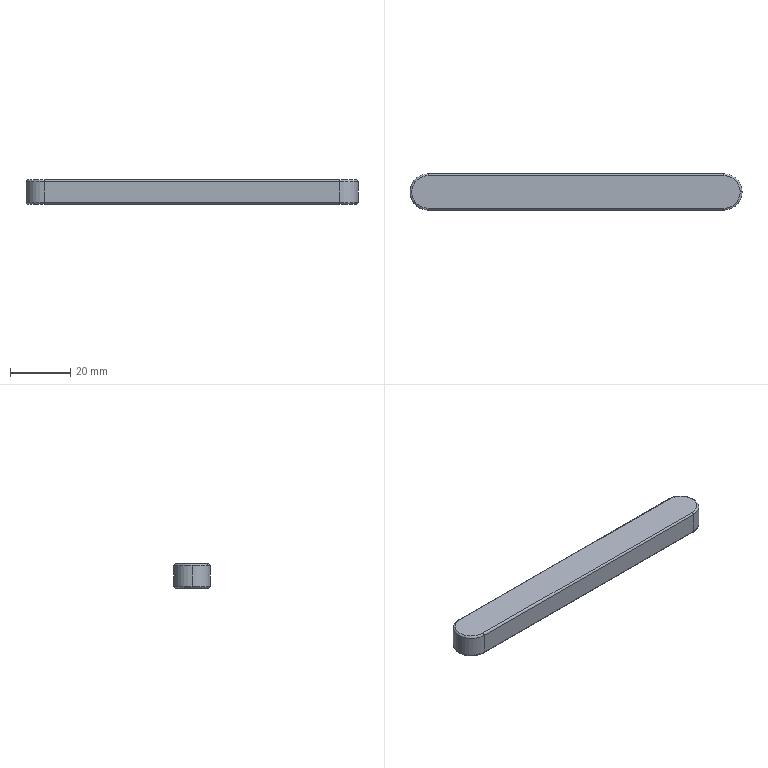Part | SolidWorks | features Extrusion 1, Fillet 1 | 1 solid | 17 faces | box 110 x 12 x 8 mm | volume 10277 mm3 | cylinder 7 | torus 6 | plane 4 | commonest cylinder face diameters 1.2 x4 12 x3
STEP:
#1=CARTESIAN_POINT('',(54.4,0.,0.));
#2=VERTEX_POINT('',#1);
#3=CARTESIAN_POINT('',(49.,-5.4,0.));
#4=VERTEX_POINT('',#3);
#5=CARTESIAN_POINT('',(49.,0.,0.));
#6=DIRECTION('',(0.,0.,-1.));
#7=DIRECTION('',(1.,0.,0.));
#8=AXIS2_PLACEMENT_3D('',#5,#6,#7);
#9=CIRCLE('',#8,5.4);
#10=EDGE_CURVE('',#2,#4,#9,.T.);
#11=ORIENTED_EDGE('',*,*,#10,.F.);
#12=CARTESIAN_POINT('',(55.,0.,0.6));
#13=VERTEX_POINT('',#12);
#14=CARTESIAN_POINT('',(54.4,0.,0.6));
#15=DIRECTION('',(0.,-1.,0.));
#16=DIRECTION('',(0.,0.,-1.));
#17=AXIS2_PLACEMENT_3D('',#14,#15,#16);
#18=CIRCLE('',#17,0.6);
#19=EDGE_CURVE('',#2,#13,#18,.T.);
#20=ORIENTED_EDGE('',*,*,#19,.T.);
#21=CARTESIAN_POINT('',(49.,-6.,0.6));
#22=VERTEX_POINT('',#21);
#23=CARTESIAN_POINT('',(49.,0.,0.6));
#24=DIRECTION('',(0.,0.,1.));
#25=DIRECTION('',(1.,0.,0.));
#26=AXIS2_PLACEMENT_3D('',#23,#24,#25);
#27=CIRCLE('',#26,6.);
#28=EDGE_CURVE('',#22,#13,#27,.T.);
#29=ORIENTED_EDGE('',*,*,#28,.F.);
#30=CARTESIAN_POINT('',(49.,-5.4,0.6));
#31=DIRECTION('',(1.,0.,0.));
#32=DIRECTION('',(0.,0.,-1.));
#33=AXIS2_PLACEMENT_3D('',#30,#31,#32);
#34=CIRCLE('',#33,0.6);
#35=EDGE_CURVE('',#22,#4,#34,.T.);
#36=ORIENTED_EDGE('',*,*,#35,.T.);
#37=EDGE_LOOP('',(#11,#20,#29,#36));
#38=FACE_OUTER_BOUND('',#37,.T.);
#39=CARTESIAN_POINT('',(49.,0.,0.6));
#40=DIRECTION('',(0.,0.,1.));
#41=DIRECTION('',(1.,0.,0.));
#42=AXIS2_PLACEMENT_3D('',#39,#40,#41);
#43=TOROIDAL_SURFACE('',#42,5.4,0.6);
#44=ADVANCED_FACE('',(#38),#43,.T.);
#45=CARTESIAN_POINT('',(55.,0.,7.4));
#46=VERTEX_POINT('',#45);
#47=CARTESIAN_POINT('',(49.,-6.,7.4));
#48=VERTEX_POINT('',#47);
#49=CARTESIAN_POINT('',(49.,0.,7.4));
#50=DIRECTION('',(0.,0.,-1.));
#51=DIRECTION('',(1.,0.,0.));
#52=AXIS2_PLACEMENT_3D('',#49,#50,#51);
#53=CIRCLE('',#52,6.);
#54=EDGE_CURVE('',#46,#48,#53,.T.);
#55=ORIENTED_EDGE('',*,*,#54,.F.);
#56=CARTESIAN_POINT('',(54.4,0.,8.));
#57=VERTEX_POINT('',#56);
#58=CARTESIAN_POINT('',(54.4,0.,7.4));
#59=DIRECTION('',(0.,-1.,0.));
#60=DIRECTION('',(0.,0.,-1.));
#61=AXIS2_PLACEMENT_3D('',#58,#59,#60);
#62=CIRCLE('',#61,0.6);
#63=EDGE_CURVE('',#46,#57,#62,.T.);
#64=ORIENTED_EDGE('',*,*,#63,.T.);
#65=CARTESIAN_POINT('',(49.,-5.4,8.));
#66=VERTEX_POINT('',#65);
#67=CARTESIAN_POINT('',(49.,0.,8.));
#68=DIRECTION('',(0.,0.,1.));
#69=DIRECTION('',(1.,0.,0.));
#70=AXIS2_PLACEMENT_3D('',#67,#68,#69);
#71=CIRCLE('',#70,5.4);
#72=EDGE_CURVE('',#66,#57,#71,.T.);
#73=ORIENTED_EDGE('',*,*,#72,.F.);
#74=CARTESIAN_POINT('',(49.,-5.4,7.4));
#75=DIRECTION('',(1.,0.,0.));
#76=DIRECTION('',(0.,0.,-1.));
#77=AXIS2_PLACEMENT_3D('',#74,#75,#76);
#78=CIRCLE('',#77,0.6);
#79=EDGE_CURVE('',#66,#48,#78,.T.);
#80=ORIENTED_EDGE('',*,*,#79,.T.);
#81=EDGE_LOOP('',(#55,#64,#73,#80));
#82=FACE_OUTER_BOUND('',#81,.T.);
#83=CARTESIAN_POINT('',(49.,0.,7.4));
#84=DIRECTION('',(0.,0.,1.));
#85=DIRECTION('',(1.,0.,0.));
#86=AXIS2_PLACEMENT_3D('',#83,#84,#85);
#87=TOROIDAL_SURFACE('',#86,5.4,0.6);
#88=ADVANCED_FACE('',(#82),#87,.T.);
#89=CARTESIAN_POINT('',(-49.,-6.,7.4));
#90=VERTEX_POINT('',#89);
#91=CARTESIAN_POINT('',(-55.,0.,7.4));
#92=VERTEX_POINT('',#91);
#93=CARTESIAN_POINT('',(-49.,0.,7.4));
#94=DIRECTION('',(0.,0.,-1.));
#95=DIRECTION('',(1.,0.,0.));
#96=AXIS2_PLACEMENT_3D('',#93,#94,#95);
#97=CIRCLE('',#96,6.);
#98=EDGE_CURVE('',#90,#92,#97,.T.);
#99=ORIENTED_EDGE('',*,*,#98,.T.);
#100=CARTESIAN_POINT('',(-55.,0.,0.6));
#101=VERTEX_POINT('',#100);
#102=CARTESIAN_POINT('',(-55.,0.,8.));
#103=DIRECTION('',(0.,0.,-1.));
#104=VECTOR('',#103,1000.);
#105=LINE('',#102,#104);
#106=EDGE_CURVE('',#92,#101,#105,.T.);
#107=ORIENTED_EDGE('',*,*,#106,.T.);
#108=CARTESIAN_POINT('',(-49.,-6.,0.6));
#109=VERTEX_POINT('',#108);
#110=CARTESIAN_POINT('',(-49.,0.,0.6));
#111=DIRECTION('',(0.,0.,1.));
#112=DIRECTION('',(1.,0.,0.));
#113=AXIS2_PLACEMENT_3D('',#110,#111,#112);
#114=CIRCLE('',#113,6.);
#115=EDGE_CURVE('',#101,#109,#114,.T.);
#116=ORIENTED_EDGE('',*,*,#115,.T.);
#117=CARTESIAN_POINT('',(-49.,-6.,8.));
#118=DIRECTION('',(0.,0.,-1.));
#119=VECTOR('',#118,1000.);
#120=LINE('',#117,#119);
#121=EDGE_CURVE('',#90,#109,#120,.T.);
#122=ORIENTED_EDGE('',*,*,#121,.F.);
#123=EDGE_LOOP('',(#99,#107,#116,#122));
#124=FACE_OUTER_BOUND('',#123,.T.);
#125=CARTESIAN_POINT('',(-49.,0.,8.));
#126=DIRECTION('',(0.,0.,-1.));
#127=DIRECTION('',(-1.,0.,0.));
#128=AXIS2_PLACEMENT_3D('',#125,#126,#127);
#129=CYLINDRICAL_SURFACE('',#128,6.);
#130=ADVANCED_FACE('',(#124),#129,.T.);
#131=ORIENTED_EDGE('',*,*,#106,.F.);
#132=CARTESIAN_POINT('',(-49.,6.,7.4));
#133=VERTEX_POINT('',#132);
#134=CARTESIAN_POINT('',(-49.,0.,7.4));
#135=DIRECTION('',(0.,0.,-1.));
#136=DIRECTION('',(1.,0.,0.));
#137=AXIS2_PLACEMENT_3D('',#134,#135,#136);
#138=CIRCLE('',#137,6.);
#139=EDGE_CURVE('',#92,#133,#138,.T.);
#140=ORIENTED_EDGE('',*,*,#139,.T.);
#141=CARTESIAN_POINT('',(-49.,6.,0.6));
#142=VERTEX_POINT('',#141);
#143=CARTESIAN_POINT('',(-49.,6.,8.));
#144=DIRECTION('',(0.,0.,-1.));
#145=VECTOR('',#144,1000.);
#146=LINE('',#143,#145);
#147=EDGE_CURVE('',#133,#142,#146,.T.);
#148=ORIENTED_EDGE('',*,*,#147,.T.);
#149=CARTESIAN_POINT('',(-49.,0.,0.6));
#150=DIRECTION('',(0.,0.,1.));
#151=DIRECTION('',(1.,0.,0.));
#152=AXIS2_PLACEMENT_3D('',#149,#150,#151);
#153=CIRCLE('',#152,6.);
#154=EDGE_CURVE('',#142,#101,#153,.T.);
#155=ORIENTED_EDGE('',*,*,#154,.T.);
#156=EDGE_LOOP('',(#131,#140,#148,#155));
#157=FACE_OUTER_BOUND('',#156,.T.);
#158=CARTESIAN_POINT('',(-49.,0.,8.));
#159=DIRECTION('',(0.,0.,-1.));
#160=DIRECTION('',(-1.,0.,0.));
#161=AXIS2_PLACEMENT_3D('',#158,#159,#160);
#162=CYLINDRICAL_SURFACE('',#161,6.);
#163=ADVANCED_FACE('',(#157),#162,.T.);
#164=CARTESIAN_POINT('',(49.,-6.,8.));
#165=DIRECTION('',(0.,0.,-1.));
#166=VECTOR('',#165,1000.);
#167=LINE('',#164,#166);
#168=EDGE_CURVE('',#48,#22,#167,.T.);
#169=ORIENTED_EDGE('',*,*,#168,.F.);
#170=CARTESIAN_POINT('',(-49.,-6.,7.4));
#171=DIRECTION('',(-1.,0.,0.));
#172=VECTOR('',#171,1000.);
#173=LINE('',#170,#172);
#174=EDGE_CURVE('',#48,#90,#173,.T.);
#175=ORIENTED_EDGE('',*,*,#174,.T.);
#176=ORIENTED_EDGE('',*,*,#121,.T.);
#177=CARTESIAN_POINT('',(-49.,-6.,0.6));
#178=DIRECTION('',(1.,0.,0.));
#179=VECTOR('',#178,1000.);
#180=LINE('',#177,#179);
#181=EDGE_CURVE('',#109,#22,#180,.T.);
#182=ORIENTED_EDGE('',*,*,#181,.T.);
#183=EDGE_LOOP('',(#169,#175,#176,#182));
#184=FACE_OUTER_BOUND('',#183,.T.);
#185=CARTESIAN_POINT('',(-49.,-6.,8.));
#186=DIRECTION('',(0.,1.,0.));
#187=DIRECTION('',(-1.,0.,0.));
#188=AXIS2_PLACEMENT_3D('',#185,#186,#187);
#189=PLANE('',#188);
#190=ADVANCED_FACE('',(#184),#189,.F.);
#191=CARTESIAN_POINT('',(49.,6.,7.4));
#192=VERTEX_POINT('',#191);
#193=CARTESIAN_POINT('',(49.,6.,0.6));
#194=VERTEX_POINT('',#193);
#195=CARTESIAN_POINT('',(49.,6.,8.));
#196=DIRECTION('',(0.,0.,-1.));
#197=VECTOR('',#196,1000.);
#198=LINE('',#195,#197);
#199=EDGE_CURVE('',#192,#194,#198,.T.);
#200=ORIENTED_EDGE('',*,*,#199,.F.);
#201=CARTESIAN_POINT('',(49.,0.,7.4));
#202=DIRECTION('',(0.,0.,-1.));
#203=DIRECTION('',(1.,0.,0.));
#204=AXIS2_PLACEMENT_3D('',#201,#202,#203);
#205=CIRCLE('',#204,6.);
#206=EDGE_CURVE('',#192,#46,#205,.T.);
#207=ORIENTED_EDGE('',*,*,#206,.T.);
#208=ORIENTED_EDGE('',*,*,#54,.T.);
#209=ORIENTED_EDGE('',*,*,#168,.T.);
#210=ORIENTED_EDGE('',*,*,#28,.T.);
#211=CARTESIAN_POINT('',(49.,0.,0.6));
#212=DIRECTION('',(0.,0.,1.));
#213=DIRECTION('',(1.,0.,0.));
#214=AXIS2_PLACEMENT_3D('',#211,#212,#213);
#215=CIRCLE('',#214,6.);
#216=EDGE_CURVE('',#13,#194,#215,.T.);
#217=ORIENTED_EDGE('',*,*,#216,.T.);
#218=EDGE_LOOP('',(#200,#207,#208,#209,#210,#217));
#219=FACE_OUTER_BOUND('',#218,.T.);
#220=CARTESIAN_POINT('',(49.,0.,8.));
#221=DIRECTION('',(0.,0.,-1.));
#222=DIRECTION('',(-1.,0.,0.));
#223=AXIS2_PLACEMENT_3D('',#220,#221,#222);
#224=CYLINDRICAL_SURFACE('',#223,6.);
#225=ADVANCED_FACE('',(#219),#224,.T.);
#226=ORIENTED_EDGE('',*,*,#147,.F.);
#227=CARTESIAN_POINT('',(49.,6.,7.4));
#228=DIRECTION('',(1.,0.,0.));
#229=VECTOR('',#228,1000.);
#230=LINE('',#227,#229);
#231=EDGE_CURVE('',#133,#192,#230,.T.);
#232=ORIENTED_EDGE('',*,*,#231,.T.);
#233=ORIENTED_EDGE('',*,*,#199,.T.);
#234=CARTESIAN_POINT('',(-49.,6.,0.6));
#235=DIRECTION('',(-1.,0.,0.));
#236=VECTOR('',#235,1000.);
#237=LINE('',#234,#236);
#238=EDGE_CURVE('',#194,#142,#237,.T.);
#239=ORIENTED_EDGE('',*,*,#238,.T.);
#240=EDGE_LOOP('',(#226,#232,#233,#239));
#241=FACE_OUTER_BOUND('',#240,.T.);
#242=CARTESIAN_POINT('',(-49.,6.,8.));
#243=DIRECTION('',(0.,-1.,0.));
#244=DIRECTION('',(1.,0.,0.));
#245=AXIS2_PLACEMENT_3D('',#242,#243,#244);
#246=PLANE('',#245);
#247=ADVANCED_FACE('',(#241),#246,.F.);
#248=CARTESIAN_POINT('',(-49.,-5.4,8.));
#249=VERTEX_POINT('',#248);
#250=CARTESIAN_POINT('',(49.,-5.4,8.));
#251=DIRECTION('',(1.,0.,0.));
#252=VECTOR('',#251,1000.);
#253=LINE('',#250,#252);
#254=EDGE_CURVE('',#249,#66,#253,.T.);
#255=ORIENTED_EDGE('',*,*,#254,.T.);
#256=ORIENTED_EDGE('',*,*,#72,.T.);
#257=CARTESIAN_POINT('',(49.,5.4,8.));
#258=VERTEX_POINT('',#257);
#259=CARTESIAN_POINT('',(49.,0.,8.));
#260=DIRECTION('',(0.,0.,1.));
#261=DIRECTION('',(1.,0.,0.));
#262=AXIS2_PLACEMENT_3D('',#259,#260,#261);
#263=CIRCLE('',#262,5.4);
#264=EDGE_CURVE('',#57,#258,#263,.T.);
#265=ORIENTED_EDGE('',*,*,#264,.T.);
#266=CARTESIAN_POINT('',(-49.,5.4,8.));
#267=VERTEX_POINT('',#266);
#268=CARTESIAN_POINT('',(-49.,5.4,8.));
#269=DIRECTION('',(-1.,0.,0.));
#270=VECTOR('',#269,1000.);
#271=LINE('',#268,#270);
#272=EDGE_CURVE('',#258,#267,#271,.T.);
#273=ORIENTED_EDGE('',*,*,#272,.T.);
#274=CARTESIAN_POINT('',(-49.,0.,8.));
#275=DIRECTION('',(0.,0.,1.));
#276=DIRECTION('',(1.,0.,0.));
#277=AXIS2_PLACEMENT_3D('',#274,#275,#276);
#278=CIRCLE('',#277,5.4);
#279=EDGE_CURVE('',#267,#249,#278,.T.);
#280=ORIENTED_EDGE('',*,*,#279,.T.);
#281=EDGE_LOOP('',(#255,#256,#265,#273,#280));
#282=FACE_OUTER_BOUND('',#281,.T.);
#283=CARTESIAN_POINT('',(-49.,0.,8.));
#284=DIRECTION('',(0.,0.,1.));
#285=DIRECTION('',(1.,0.,0.));
#286=AXIS2_PLACEMENT_3D('',#283,#284,#285);
#287=PLANE('',#286);
#288=ADVANCED_FACE('',(#282),#287,.T.);
#289=CARTESIAN_POINT('',(-49.,5.4,0.));
#290=VERTEX_POINT('',#289);
#291=CARTESIAN_POINT('',(49.,5.4,0.));
#292=VERTEX_POINT('',#291);
#293=CARTESIAN_POINT('',(-49.,5.4,0.));
#294=DIRECTION('',(1.,0.,0.));
#295=VECTOR('',#294,1000.);
#296=LINE('',#293,#295);
#297=EDGE_CURVE('',#290,#292,#296,.T.);
#298=ORIENTED_EDGE('',*,*,#297,.T.);
#299=CARTESIAN_POINT('',(49.,0.,0.));
#300=DIRECTION('',(0.,0.,-1.));
#301=DIRECTION('',(1.,0.,0.));
#302=AXIS2_PLACEMENT_3D('',#299,#300,#301);
#303=CIRCLE('',#302,5.4);
#304=EDGE_CURVE('',#292,#2,#303,.T.);
#305=ORIENTED_EDGE('',*,*,#304,.T.);
#306=ORIENTED_EDGE('',*,*,#10,.T.);
#307=CARTESIAN_POINT('',(-49.,-5.4,0.));
#308=VERTEX_POINT('',#307);
#309=CARTESIAN_POINT('',(-49.,-5.4,0.));
#310=DIRECTION('',(-1.,0.,0.));
#311=VECTOR('',#310,1000.);
#312=LINE('',#309,#311);
#313=EDGE_CURVE('',#4,#308,#312,.T.);
#314=ORIENTED_EDGE('',*,*,#313,.T.);
#315=CARTESIAN_POINT('',(-49.,0.,0.));
#316=DIRECTION('',(0.,0.,-1.));
#317=DIRECTION('',(1.,0.,0.));
#318=AXIS2_PLACEMENT_3D('',#315,#316,#317);
#319=CIRCLE('',#318,5.4);
#320=EDGE_CURVE('',#308,#290,#319,.T.);
#321=ORIENTED_EDGE('',*,*,#320,.T.);
#322=EDGE_LOOP('',(#298,#305,#306,#314,#321));
#323=FACE_OUTER_BOUND('',#322,.T.);
#324=CARTESIAN_POINT('',(-49.,0.,0.));
#325=DIRECTION('',(0.,0.,1.));
#326=DIRECTION('',(1.,0.,0.));
#327=AXIS2_PLACEMENT_3D('',#324,#325,#326);
#328=PLANE('',#327);
#329=ADVANCED_FACE('',(#323),#328,.F.);
#330=CARTESIAN_POINT('',(-49.,5.4,7.4));
#331=DIRECTION('',(1.,0.,0.));
#332=DIRECTION('',(0.,0.,-1.));
#333=AXIS2_PLACEMENT_3D('',#330,#331,#332);
#334=CIRCLE('',#333,0.6);
#335=EDGE_CURVE('',#133,#267,#334,.T.);
#336=ORIENTED_EDGE('',*,*,#335,.F.);
#337=ORIENTED_EDGE('',*,*,#139,.F.);
#338=ORIENTED_EDGE('',*,*,#98,.F.);
#339=CARTESIAN_POINT('',(-49.,-5.4,7.4));
#340=DIRECTION('',(1.,0.,0.));
#341=DIRECTION('',(0.,0.,-1.));
#342=AXIS2_PLACEMENT_3D('',#339,#340,#341);
#343=CIRCLE('',#342,0.6);
#344=EDGE_CURVE('',#249,#90,#343,.T.);
#345=ORIENTED_EDGE('',*,*,#344,.F.);
#346=ORIENTED_EDGE('',*,*,#279,.F.);
#347=EDGE_LOOP('',(#336,#337,#338,#345,#346));
#348=FACE_OUTER_BOUND('',#347,.T.);
#349=CARTESIAN_POINT('',(-49.,0.,7.4));
#350=DIRECTION('',(0.,0.,1.));
#351=DIRECTION('',(1.,0.,0.));
#352=AXIS2_PLACEMENT_3D('',#349,#350,#351);
#353=TOROIDAL_SURFACE('',#352,5.4,0.6);
#354=ADVANCED_FACE('',(#348),#353,.T.);
#355=ORIENTED_EDGE('',*,*,#344,.T.);
#356=ORIENTED_EDGE('',*,*,#174,.F.);
#357=ORIENTED_EDGE('',*,*,#79,.F.);
#358=ORIENTED_EDGE('',*,*,#254,.F.);
#359=EDGE_LOOP('',(#355,#356,#357,#358));
#360=FACE_OUTER_BOUND('',#359,.T.);
#361=CARTESIAN_POINT('',(-49.,-5.4,7.4));
#362=DIRECTION('',(-1.,0.,0.));
#363=DIRECTION('',(0.,-1.,0.));
#364=AXIS2_PLACEMENT_3D('',#361,#362,#363);
#365=CYLINDRICAL_SURFACE('',#364,0.6);
#366=ADVANCED_FACE('',(#360),#365,.T.);
#367=ORIENTED_EDGE('',*,*,#335,.T.);
#368=ORIENTED_EDGE('',*,*,#272,.F.);
#369=CARTESIAN_POINT('',(49.,5.4,7.4));
#370=DIRECTION('',(1.,0.,0.));
#371=DIRECTION('',(0.,0.,-1.));
#372=AXIS2_PLACEMENT_3D('',#369,#370,#371);
#373=CIRCLE('',#372,0.6);
#374=EDGE_CURVE('',#192,#258,#373,.T.);
#375=ORIENTED_EDGE('',*,*,#374,.F.);
#376=ORIENTED_EDGE('',*,*,#231,.F.);
#377=EDGE_LOOP('',(#367,#368,#375,#376));
#378=FACE_OUTER_BOUND('',#377,.T.);
#379=CARTESIAN_POINT('',(-49.,5.4,7.4));
#380=DIRECTION('',(1.,0.,0.));
#381=DIRECTION('',(0.,1.,0.));
#382=AXIS2_PLACEMENT_3D('',#379,#380,#381);
#383=CYLINDRICAL_SURFACE('',#382,0.6);
#384=ADVANCED_FACE('',(#378),#383,.T.);
#385=ORIENTED_EDGE('',*,*,#63,.F.);
#386=ORIENTED_EDGE('',*,*,#206,.F.);
#387=ORIENTED_EDGE('',*,*,#374,.T.);
#388=ORIENTED_EDGE('',*,*,#264,.F.);
#389=EDGE_LOOP('',(#385,#386,#387,#388));
#390=FACE_OUTER_BOUND('',#389,.T.);
#391=CARTESIAN_POINT('',(49.,0.,7.4));
#392=DIRECTION('',(0.,0.,1.));
#393=DIRECTION('',(1.,0.,0.));
#394=AXIS2_PLACEMENT_3D('',#391,#392,#393);
#395=TOROIDAL_SURFACE('',#394,5.4,0.6);
#396=ADVANCED_FACE('',(#390),#395,.T.);
#397=CARTESIAN_POINT('',(-49.,5.4,0.6));
#398=DIRECTION('',(1.,0.,0.));
#399=DIRECTION('',(0.,0.,-1.));
#400=AXIS2_PLACEMENT_3D('',#397,#398,#399);
#401=CIRCLE('',#400,0.6);
#402=EDGE_CURVE('',#290,#142,#401,.T.);
#403=ORIENTED_EDGE('',*,*,#402,.F.);
#404=ORIENTED_EDGE('',*,*,#320,.F.);
#405=CARTESIAN_POINT('',(-49.,-5.4,0.6));
#406=DIRECTION('',(1.,0.,0.));
#407=DIRECTION('',(0.,0.,-1.));
#408=AXIS2_PLACEMENT_3D('',#405,#406,#407);
#409=CIRCLE('',#408,0.6);
#410=EDGE_CURVE('',#109,#308,#409,.T.);
#411=ORIENTED_EDGE('',*,*,#410,.F.);
#412=ORIENTED_EDGE('',*,*,#115,.F.);
#413=ORIENTED_EDGE('',*,*,#154,.F.);
#414=EDGE_LOOP('',(#403,#404,#411,#412,#413));
#415=FACE_OUTER_BOUND('',#414,.T.);
#416=CARTESIAN_POINT('',(-49.,0.,0.6));
#417=DIRECTION('',(0.,0.,1.));
#418=DIRECTION('',(1.,0.,0.));
#419=AXIS2_PLACEMENT_3D('',#416,#417,#418);
#420=TOROIDAL_SURFACE('',#419,5.4,0.6);
#421=ADVANCED_FACE('',(#415),#420,.T.);
#422=ORIENTED_EDGE('',*,*,#410,.T.);
#423=ORIENTED_EDGE('',*,*,#313,.F.);
#424=ORIENTED_EDGE('',*,*,#35,.F.);
#425=ORIENTED_EDGE('',*,*,#181,.F.);
#426=EDGE_LOOP('',(#422,#423,#424,#425));
#427=FACE_OUTER_BOUND('',#426,.T.);
#428=CARTESIAN_POINT('',(-49.,-5.4,0.6));
#429=DIRECTION('',(1.,0.,0.));
#430=DIRECTION('',(0.,1.,0.));
#431=AXIS2_PLACEMENT_3D('',#428,#429,#430);
#432=CYLINDRICAL_SURFACE('',#431,0.6);
#433=ADVANCED_FACE('',(#427),#432,.T.);
#434=ORIENTED_EDGE('',*,*,#402,.T.);
#435=ORIENTED_EDGE('',*,*,#238,.F.);
#436=CARTESIAN_POINT('',(49.,5.4,0.6));
#437=DIRECTION('',(1.,0.,0.));
#438=DIRECTION('',(0.,0.,-1.));
#439=AXIS2_PLACEMENT_3D('',#436,#437,#438);
#440=CIRCLE('',#439,0.6);
#441=EDGE_CURVE('',#292,#194,#440,.T.);
#442=ORIENTED_EDGE('',*,*,#441,.F.);
#443=ORIENTED_EDGE('',*,*,#297,.F.);
#444=EDGE_LOOP('',(#434,#435,#442,#443));
#445=FACE_OUTER_BOUND('',#444,.T.);
#446=CARTESIAN_POINT('',(-49.,5.4,0.6));
#447=DIRECTION('',(-1.,0.,0.));
#448=DIRECTION('',(0.,-1.,0.));
#449=AXIS2_PLACEMENT_3D('',#446,#447,#448);
#450=CYLINDRICAL_SURFACE('',#449,0.6);
#451=ADVANCED_FACE('',(#445),#450,.T.);
#452=ORIENTED_EDGE('',*,*,#19,.F.);
#453=ORIENTED_EDGE('',*,*,#304,.F.);
#454=ORIENTED_EDGE('',*,*,#441,.T.);
#455=ORIENTED_EDGE('',*,*,#216,.F.);
#456=EDGE_LOOP('',(#452,#453,#454,#455));
#457=FACE_OUTER_BOUND('',#456,.T.);
#458=CARTESIAN_POINT('',(49.,0.,0.6));
#459=DIRECTION('',(0.,0.,1.));
#460=DIRECTION('',(1.,0.,0.));
#461=AXIS2_PLACEMENT_3D('',#458,#459,#460);
#462=TOROIDAL_SURFACE('',#461,5.4,0.6);
#463=ADVANCED_FACE('',(#457),#462,.T.);
#464=CLOSED_SHELL('',(#44,#88,#130,#163,#190,#225,#247,#288,#329,#354,#366,#384,#396,#421,#433,#451,#463));
#465=MANIFOLD_SOLID_BREP('',#464);
#466=CARTESIAN_POINT('',(0.,0.,0.));
#467=DIRECTION('',(0.,0.,1.));
#468=DIRECTION('',(1.,0.,0.));
#469=AXIS2_PLACEMENT_3D('',#466,#467,#468);
#470=(LENGTH_UNIT()NAMED_UNIT(*)SI_UNIT(.MILLI.,.METRE.));
#471=UNCERTAINTY_MEASURE_WITH_UNIT(LENGTH_MEASURE(0.00001),#470,'','');
#472=(NAMED_UNIT(*)PLANE_ANGLE_UNIT()SI_UNIT($,.RADIAN.));
#473=(NAMED_UNIT(*)SI_UNIT($,.STERADIAN.)SOLID_ANGLE_UNIT());
#474=(GEOMETRIC_REPRESENTATION_CONTEXT(3)GLOBAL_UNCERTAINTY_ASSIGNED_CONTEXT((#471))GLOBAL_UNIT_ASSIGNED_CONTEXT((#470,#472,#473))REPRESENTATION_CONTEXT('',''));
#475=ADVANCED_BREP_SHAPE_REPRESENTATION('',(#465,#469),#474);